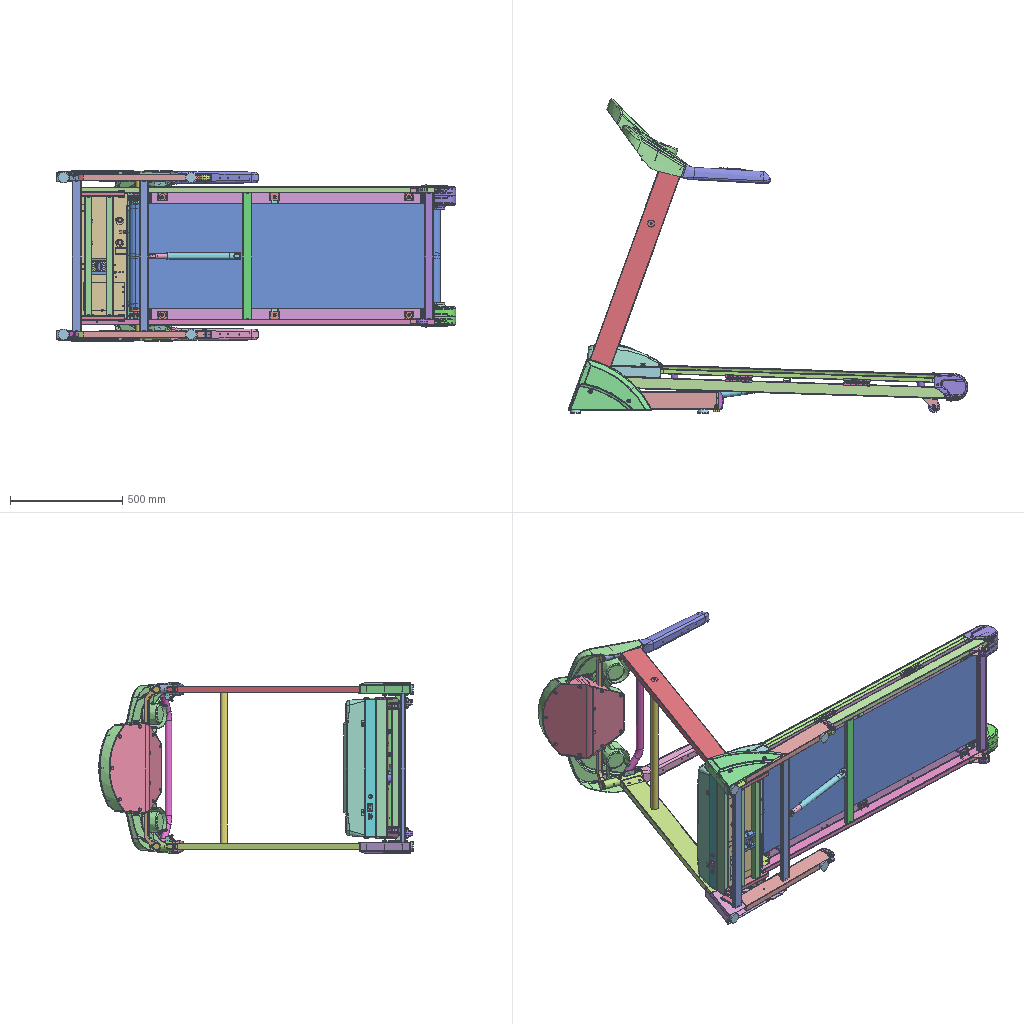Assembly | STEP file | 109 different items | 222 placed | box 1782 x 1401 x 762 mm
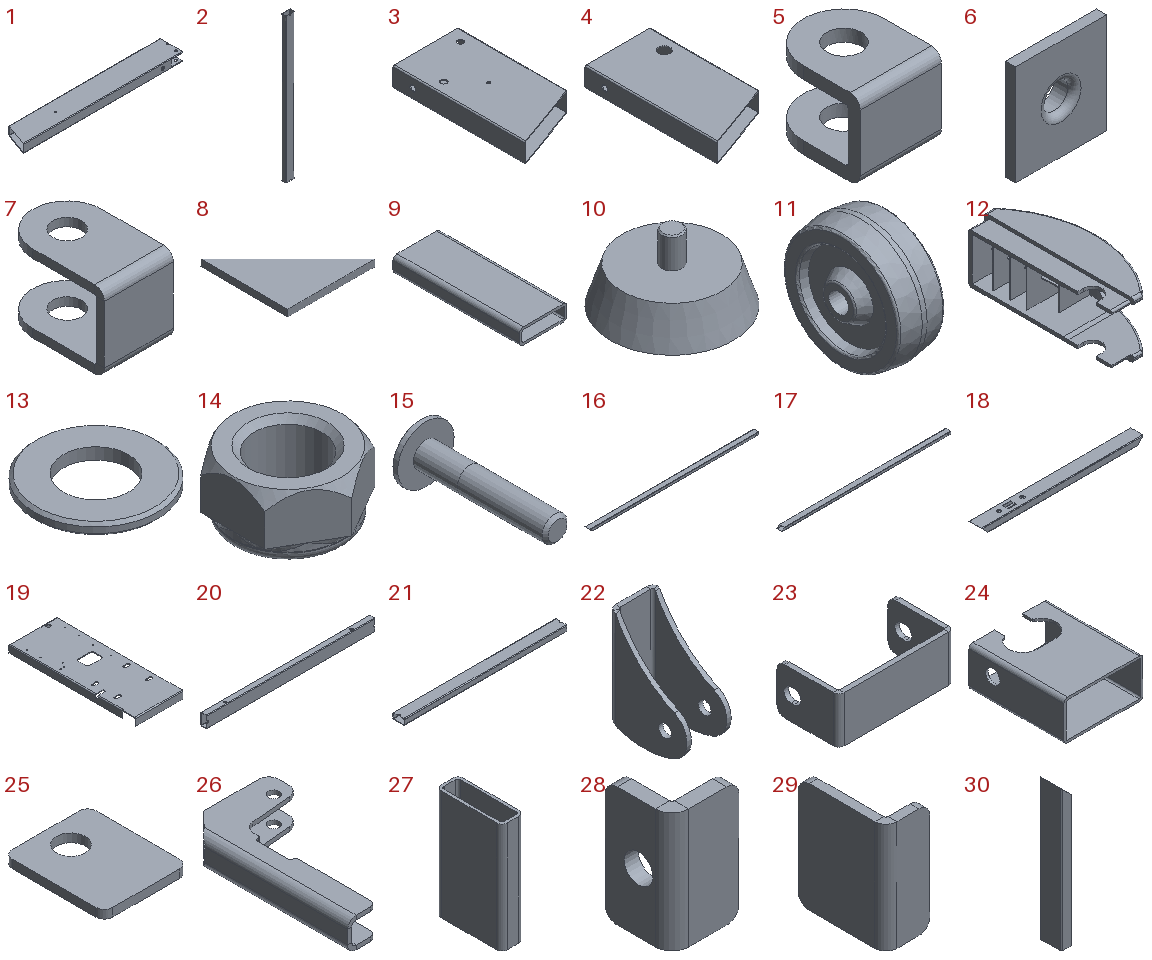Parts list (item | name | quantity | parent item | size | volume):
1 | 7100101 | x2 | in 7100100 | 550 x 80 x 30 mm | 167922 mm3
2 | 7100102 | x2 | in 7100100 | 40 x 20 x 670 mm | 111433 mm3
3 | PN_0021 | x1 | in 7100100 | 100 x 200 x 30 mm | 68376 mm3
4 | PN_0060 | x1 | in 7100100 | 100 x 200 x 30 mm | 68036 mm3
5 | PN_0076_default | x1 | in 7100100 | 20 x 24 x 19 mm | 3011 mm3
6 | 7100105 | x2 | in 7100100 | 27 x 6 x 30 mm | 2422 mm3
7 | 7100106 | x4 | in 7100100, 7100500 | 25 x 38.5 x 28 mm | 6374 mm3
8 | 7100107 | x4 | in 7100100 | 40 x 40 x 3 mm | 2400 mm3
9 | 7100109 | x2 | in 7100100 | 30 x 80 x 10 mm | 8519 mm3
10 | 7100103W | x4 | in PN_0072 | 48.954 x 48.954 x 27.5 mm | 24706 mm3
11 | PN_0027 | x1 | in PN_0072 | 22 x 52.843 x 52.843 mm | 34026 mm3
12 | 7100102W | x2 | in PN_0072 | 30 x 80 x 30 mm | 16145 mm3
13 | PN_0069 | x7 | in PN_0072, PN_0095 | 17 x 17 x 1.6 mm | 252.969 mm3
14 | PN_0039 | x4 | in PN_0072, PN_0095 | 13.017 x 15.011 x 7.5 mm | 666.866 mm3
15 | PN_0065 | x4 | in PN_0072, PN_0095 | 18 x 46.451 x 18 mm | 2805 mm3
16 | PN_0068 | x1 | in 7100500 | 1650 x 50 x 25 mm | 346400 mm3
17 | PN_0073 | x1 | in 7100500 | 1650 x 50 x 25 mm | 346388 mm3
18 | 7100502 | x1 | in 7100500 | 613 x 50 x 25 mm | 116984 mm3
19 | PN_0081_default | x1 | in 7100500 | 210 x 564 x 33 mm | 418851 mm3
20 | 7100504 | x1 | in 7100500 | 565 x 20 x 40 mm | 94145 mm3
21 | 7100505 | x1 | in 7100500 | 565 x 40 x 20 mm | 93951 mm3
22 | 7100506 | x2 | in 7100500 | 30 x 53 x 70.522 mm | 17329 mm3
23 | 7100507 | x2 | in 7100500 | 75 x 40 x 30 mm | 12701 mm3
24 | 7100508 | x1 | in 7100500 | 50 x 60 x 25 mm | 11554 mm3
25 | 7100509 | x1 | in 7100500 | 50 x 60 x 5 mm | 13731 mm3
26 | 7100510 | x1 | in 7100500 | 84 x 160 x 29 mm | 53248 mm3
27 | 7100511 | x2 | in 7100500 | 10 x 30 x 50 mm | 4316 mm3
28 | 7100513 | x4 | in 7100500 | 14 x 14 x 25 mm | 1710 mm3
29 | 7100514 | x2 | in 7100500 | 10 x 20 x 25 mm | 1357 mm3
30 | 7100515 | x1 | in 7100500 | 25 x 50 x 325 mm | 66092 mm3
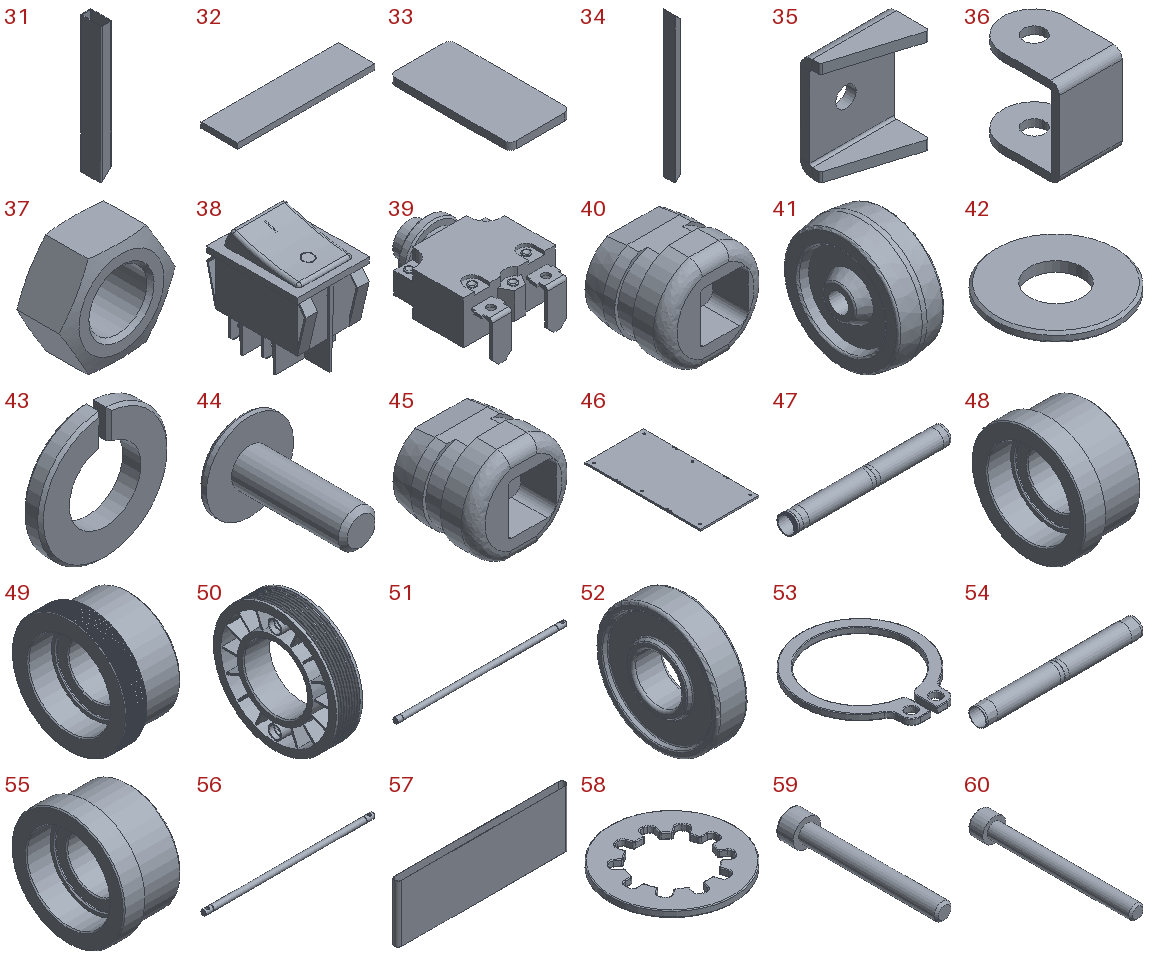31 | 7100516 | x1 | in 7100500 | 25 x 50 x 325 mm | 65710 mm3
32 | 7100517 | x2 | in 7100500 | 75 x 20 x 3 mm | 4500 mm3
33 | 7100518 | x2 | in 7100500 | 25 x 50 x 3 mm | 3734 mm3
34 | 7100519 | x1 | in 7100500 | 25 x 50 x 613 mm | 124358 mm3
35 | 7100520 | x6 | in 7100500 | 35 x 18.649 x 43 mm | 8130 mm3
36 | 7100521 | x1 | in 7100500 | 25 x 35 x 35 mm | 6553 mm3
37 | PN_0091 | x19 | in 7100500, 7101200, PN_0017, PN_0018 | 16 x 7 x 13.856 mm | 779.97 mm3
38 | EP002 | x1 | in PN_0095 | 25 x 34.5 x 34.784 mm | 14567 mm3
39 | EC002 | x1 | in PN_0095 | 29.3 x 39.3 x 19.65 mm | 10331 mm3
40 | PN_0075_default | x1 | in PN_0095 | 17 x 14 x 16 mm | 1519 mm3
41 | PN_0036 | x2 | in PN_0095 | 22 x 52.843 x 52.843 mm | 34026 mm3
42 | PN_0057 | x6 | in PN_0095 | 9.8 x 9.8 x 0.8 mm | 48.045 mm3
43 | PN_0080 | x5 | in PN_0095 | 9.2 x 1.3 x 9.193 mm | 57.255 mm3
44 | PN_0093 | x8 | in PN_0095 | 9.4 x 14.503 x 9.4 mm | 245.335 mm3
45 | PN_0096_default | x1 | in PN_0095 | 17 x 14 x 16 mm | 1519 mm3
46 | DECAK 601 | x1 | in PN_0095 | 605 x 1200 x 18 mm | 13042894 mm3
47 | PN_0083_default | x1 | in PN_0022 | 495 x 56 x 56 mm | 244128 mm3
48 | PN_0001_default | x1 | in PN_0022 | 30 x 55.001 x 55.001 mm | 38129 mm3
49 | PN_0034_default | x1 | in PN_0022 | 30 x 55.999 x 56 mm | 38879 mm3
50 | PN_0025_default | x1 | in PN_0022 | 23 x 108.001 x 108.001 mm | 96628 mm3
51 | 7100702 | x1 | in PN_0038 | 565 x 17 x 17 mm | 128589 mm3
52 | PL6203ZZA_default | x4 | in PN_0038, PN_0026 | 11 x 44 x 44 mm | 11669 mm3
53 | PN_0084 | x4 | in PN_0038, PN_0026 | 19 x 21.5 x 1 mm | 101.865 mm3
54 | PN_0050_default | x1 | in PN_0078 | 485 x 56 x 56 mm | 236794 mm3
55 | PN_0003_default | x2 | in PN_0078 | 30 x 54.43 x 54.43 mm | 37639 mm3
56 | 7100803 | x1 | in PN_0026 | 560 x 17 x 17 mm | 125657 mm3
57 | RUBE 601 | x1 | in PN_0095 | 1389 x 59.2 x 465 mm | 2113671 mm3
58 | PN_0023 | x3 | in PN_0095 | 15 x 15 x 0.8 mm | 82.689 mm3
59 | PN_0020 | x1 | in PN_0095 | 13 x 73 x 13 mm | 4160 mm3
60 | PN_0049 | x2 | in PN_0095 | 13 x 88 x 13 mm | 4914 mm3
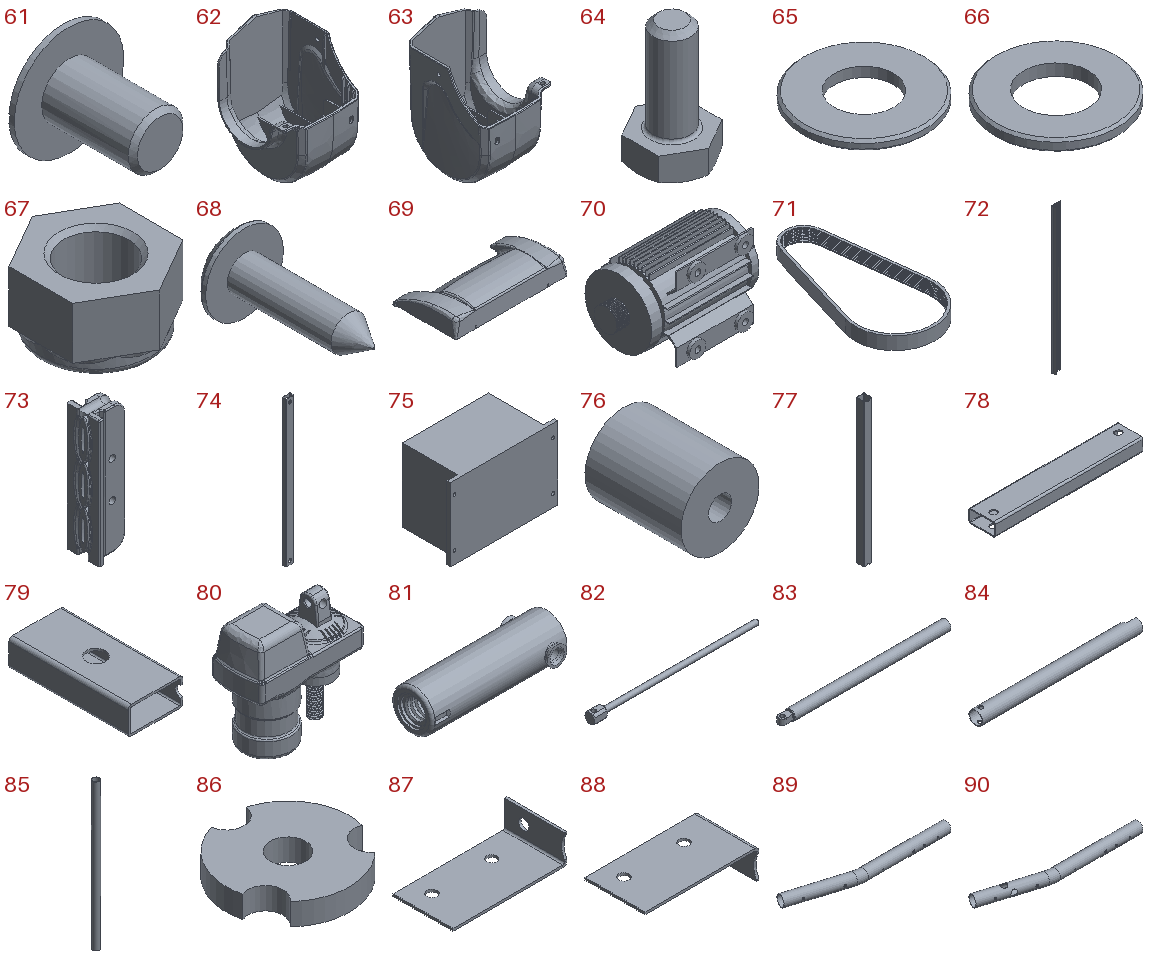61 | PN_0016 | x3 | in PN_0095 | 12 x 12.352 x 12 mm | 428.238 mm3
62 | EDN CAP 601L | x1 | in PN_0095 | - | 183620 mm3
63 | EDN CAP 601R | x1 | in PN_0095 | - | 183322 mm3
64 | PN_0058_M10 | x4 | in PN_0095 | 17 x 19.6 x 32 mm | 3678 mm3
65 | PN_0085 | x4 | in PN_0095 | 25 x 25 x 2 mm | 736.18 mm3
66 | PN_0092 | x4 | in PN_0095 | 21 x 21 x 2 mm | 492.233 mm3
67 | PN_0090 | x4 | in PN_0095 | 17 x 19.63 x 10.5 mm | 1722 mm3
68 | PN_0011 | x2 | in PN_0095 | 9 x 17.646 x 9 mm | 255.973 mm3
69 | 96L | x1 | in PN_0095 | - | -
70 | AC MOTOR 1.5KW | x1 | in PN_0095 | 263.5 x 156.005 x 174 mm | 3095920 mm3
71 | DE200JS8 | x1 | in PN_0095 | 111 x 221.3 x 18 mm | 22925 mm3
72 | SIDE | x2 | in PN_0095 | 76 x 36.5 x 1230 mm | 490001 mm3
73 | jianzhendian | x2 | in PN_0095 | 30 x 30 x 117 mm | 56101 mm3
74 | 7100901 | x1 | in PN_0095 | 30 x 15 x 555 mm | 54621 mm3
75 | Inverter | x1 | in PN_0095 | 185 x 101 x 126 mm | 1922919 mm3
76 | DECH02 | x4 | in PN_0095 | 30 x 37 x 30 mm | 23800 mm3
77 | PN_0043_default | x2 | in 7100400 | 30 x 30 x 532 mm | 88457 mm3
78 | 7100402 | x2 | in 7100400 | 225 x 40 x 20 mm | 36971 mm3
79 | 7100403 | x2 | in 7100400 | 30 x 65 x 15 mm | 6216 mm3
80 | J09 601A_default | x1 | in 710 | 148.1 x 70.5 x 151.812 mm | 777031 mm3
81 | J09 601B | x1 | in 710 | 115 x 41.999 x 35 mm | 49295 mm3
82 | GAS SHOCK 609S | x1 | in 710 | 353.5 x 20 x 20 mm | 34694 mm3
83 | GAS SHOCK 609X | x1 | in 710 | 359 x 22 x 22 mm | 94119 mm3
84 | GAS SHOCK 610W | x1 | in 710 | 330 x 28 x 28 mm | 39789 mm3
85 | 7101301 | x1 | in 7101300 | 31.8 x 31.8 x 725 mm | 103519 mm3
86 | PN_0051_default | x2 | in 7101300 | 28 x 27.429 x 5 mm | 2473 mm3
87 | PN_0007 | x1 | in 7101200 | 95 x 50 x 24.5 mm | 11238 mm3
88 | PN_0031 | x1 | in 7101200 | 95 x 50 x 24.5 mm | 11238 mm3
89 | PN_0002 | x1 | in 7101200 | 530.631 x 103.035 x 38.1 mm | 88866 mm3
90 | PN_0042 | x1 | in 7101200 | 530.631 x 103.035 x 38.1 mm | 88372 mm3
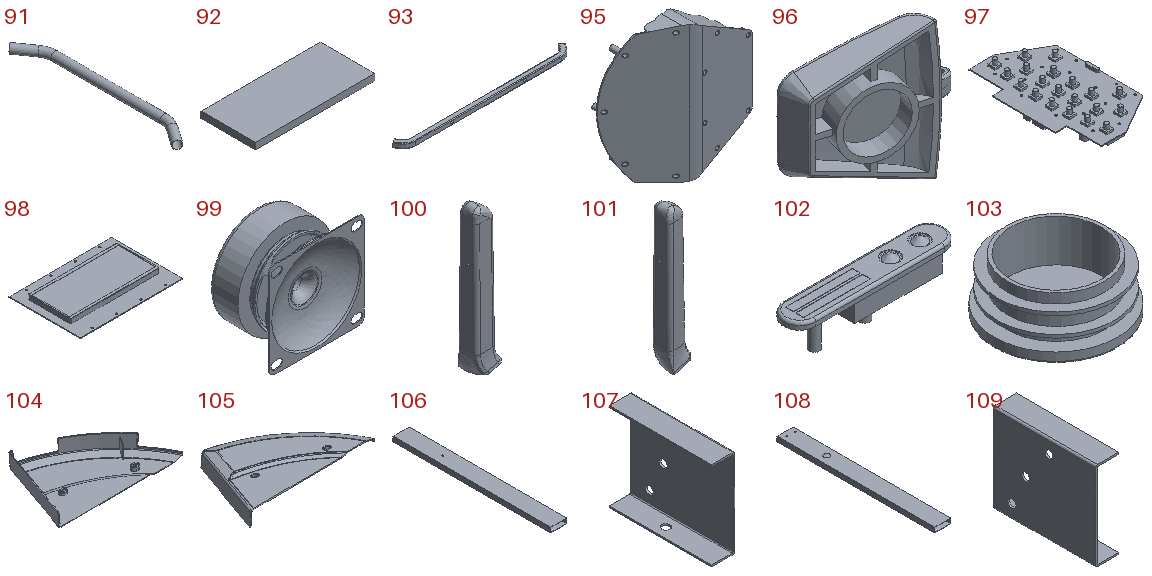91 | 7101203 | x1 | in 7101200 | 89.278 x 660.628 x 31.8 mm | 96707 mm3
92 | 7101204 | x2 | in 7101200 | 55 x 25 x 3 mm | 4125 mm3
93 | 7101205 | x1 | in 7101200 | 697.147 x 49.49 x 20 mm | 75230 mm3
94 | NA609S-A | x1 | in NA609SZ | - | -
95 | NA609S-B | x1 | in NA609SZ | 340.609 x 142.904 x 405.431 mm | 455741 mm3
96 | NA609S-C | x1 | in NA609SZ | 35.148 x 15.37 x 38.312 mm | 3411 mm3
97 | PCB Plate-618 | x1 | in NA609SZ | 132 x 230 x 23.4 mm | 58668 mm3
98 | - | x1 | in NA609SZ | 210 x 145 x 11 mm | 188408 mm3
99 | - | x2 | in NA609SZ | 50 x 31.5 x 50 mm | 33375 mm3
100 | PN_0006 | x1 | in PN_0061 | 71.872 x 63.257 x 397.874 mm | 548309 mm3
101 | PN_0048 | x1 | in PN_0061 | 71.871 x 63.257 x 397.874 mm | 548109 mm3
102 | 7101207W | x2 | in PN_0061 | 119.5 x 24 x 32.509 mm | 28513 mm3
103 | 7101208W | x2 | in PN_0061 | 38 x 38 x 16 mm | 5202 mm3
104 | Right column cover | x1 | in 710 | 372.789 x 229.022 x 48 mm | 179177 mm3
105 | Left column cover | x1 | in 710 | 372.789 x 229.022 x 48 mm | 179176 mm3
106 | PN_0071 | x1 | in PN_0017 | 100 x 950 x 30 mm | 355925 mm3
107 | PN_0066 | x1 | in PN_0017 | 25 x 110 x 95 mm | 29808 mm3
108 | PN_0087 | x1 | in PN_0018 | 100 x 950 x 30 mm | 355925 mm3
109 | PN_0012 | x1 | in PN_0018 | 25 x 110 x 95 mm | 29808 mm3
Placements (level | parent | child | x y z in mm | rotation matrix by rows):
1 | 710 | PN_0072 | 319.734 -99.186 350.0 | 1 0 0 0 1 0 0 0 1
2 | PN_0072 | 7100100 | -0.0 -0.0 -0.0 | 1 0 0 0 1 0 0 0 1
3 | 7100100 | 7100101 | -0.0 -0.0 -0.0 | 1 0 0 0 1 0 0 0 1
3 | 7100100 | 7100101 | -0.0 -0.0 -700.0 | 1 0 0 0 1 0 0 0 1
3 | 7100100 | 7100102 | -280.0 20.0 -350.0 | 1 0 0 0 1 0 0 0 1
3 | 7100100 | 7100102 | -580.0 20.0 -350.0 | 1 0 0 0 1 0 0 0 1
3 | 7100100 | PN_0021 | -609.433 -17.101 -0.0 | 0.9397 0.342 0 -0.342 0.9397 0 0 0 1
3 | 7100100 | PN_0060 | -609.433 -17.101 -700.0 | 0.9397 0.342 0 -0.342 0.9397 0 0 0 1
3 | 7100100 | PN_0076_default | -260.0 30.0 -350.0 | 0 1 0 -1 0 0 0 0 1
3 | 7100100 | 7100105 | -638.73 0.0 0.0 | 0 0 -1 0 1 0 1 0 -0
3 | 7100100 | 7100105 | -638.73 0.0 -700.0 | 0 0 1 0 1 0 -1 0 0
3 | 7100100 | 7100106 | -580.0 40.0 -74.0 | 1 0 0 0 1 0 0 0 1
3 | 7100100 | 7100106 | -580.0 40.0 -626.0 | 1 0 0 0 1 0 0 0 1
3 | 7100100 | 7100107 | -560.0 80.0 -685.0 | 0 0 -1 0 1 0 1 0 0
3 | 7100100 | 7100107 | -563.0 80.0 -15.0 | 0 0 1 0 1 0 -1 0 0
3 | 7100100 | 7100107 | -281.5 80.0 -15.0 | 0 0 1 0 1 0 -1 0 0
3 | 7100100 | 7100107 | -281.5 40.0 -645.0 | 0 0 1 1 0 0 0 1 -0
3 | 7100100 | 7100109 | -599.674 40.0 -672.775 | 1 0 0 0 1 0 0 0 1
3 | 7100100 | 7100109 | -599.674 40.0 -12.775 | 1 0 0 0 1 0 0 0 1
2 | PN_0072 | 7100103W | -638.73 0.0 -0.0 | 0.9991 -0.04147 0 0 0 1 -0.04147 -0.9991 0
2 | PN_0072 | 7100103W | -70.0 -0.0 0.0 | -0.9344 0.3562 0 0 0 1 0.3562 0.9344 0
2 | PN_0072 | PN_0027 | -10.0 15.0 -0.0 | 0 0 1 0 1 0 -1 0 0
2 | PN_0072 | 7100102W | -0.0 40.0 -0.0 | 1 0 0 0 1 0 0 0 1
2 | PN_0072 | PN_0069 | -10.0 15.0 -16.6 | 1 0 0 0 1 0 0 0 1
2 | PN_0072 | PN_0069 | -10.0 15.0 -683.4 | -0.9237 -0.383 0 -0.383 0.9237 0 0 0 -1
2 | PN_0072 | PN_0039 | -10.0 15.0 -22.1 | 1 0 0 0 1 0 0 0 1
2 | PN_0072 | PN_0039 | -10.0 15.0 -677.9 | -0.9237 -0.383 0 -0.383 0.9237 0 0 0 -1
2 | PN_0072 | PN_0065 | -10.0 15.0 15.0 | 1 0 0 0 0 -1 0 1 0
2 | PN_0072 | PN_0065 | -10.0 15.0 -715.0 | 1 0 0 0 0 1 0 -1 0
2 | PN_0072 | 7100103W | -638.73 0.0 -700.0 | 0.9991 -0.04147 0 0 0 1 -0.04147 -0.9991 0
2 | PN_0072 | 7100103W | -70.0 -0.0 -700.0 | -0.9344 0.3562 0 0 0 1 0.3562 0.9344 0
2 | PN_0072 | 7100102W | -0.0 40.0 -700.0 | 1 0 0 0 1 0 0 0 1
1 | 710 | PN_0095 | 446.175 68.129 310.459 | 0.9995 0.03221 0 -0.03221 0.9995 0 0 0 1
2 | PN_0095 | 7100500 | -0.0 -0.0 -0.0 | 1 0 0 0 1 0 0 0 1
3 | 7100500 | PN_0068 | 112.255 -64.436 -15.459 | 1 0 0 0 1 0 0 0 1
3 | 7100500 | PN_0073 | 112.255 -64.436 -605.459 | 1 0 0 0 1 0 0 0 1
3 | 7100500 | 7100502 | -700.245 -14.436 -310.459 | 0 0 -1 0 1 0 1 0 0
3 | 7100500 | PN_0081_default | -687.745 -86.436 -310.459 | -1 0 0 0 0 -1 0 -1 0
3 | 7100500 | 7100504 | 867.255 -79.436 -310.459 | 0 0 1 0 1 0 -1 0 -0
3 | 7100500 | 7100505 | 57.255 -79.436 -310.459 | 0 -1 0 0 0 -1 1 0 0
3 | 7100500 | 7100506 | 825.755 -89.436 -17.959 | 0 0 -1 0 1 0 1 0 0
3 | 7100500 | 7100506 | 825.755 -89.436 -602.959 | 0 0 -1 0 1 0 1 0 0
3 | 7100500 | 7100507 | 899.755 -24.436 -32.959 | 1 0 0 0 0 1 0 -1 0
3 | 7100500 | 7100507 | 899.755 -24.436 -587.959 | 1 0 0 0 0 -1 0 1 -0
3 | 7100500 | 7100508 | -442.745 -39.436 -580.459 | 1 0 0 0 1 0 0 0 1
3 | 7100500 | 7100509 | -442.745 -69.436 -32.959 | 1 0 0 0 1 0 0 0 1
3 | 7100500 | 7100510 | -666.745 73.564 -357.459 | 1 0 0 0 1 0 0 0 1
3 | 7100500 | 7100511 | -505.745 -137.337 -301.977 | 0 0 1 -1 0 0 0 -1 0
3 | 7100500 | 7100511 | -662.745 -25.535 -109.977 | 0 0 -1 1 0 0 0 -1 -0
3 | 7100500 | 7100513 | -465.745 10.564 -614.959 | 0 0 -1 0 1 0 1 0 0
3 | 7100500 | 7100513 | -712.745 10.564 -112.959 | 1 0 0 0 1 0 0 0 1
3 | 7100500 | 7100513 | -465.745 10.564 -5.959 | 0 0 1 0 1 0 -1 0 0
3 | 7100500 | 7100513 | -712.745 10.564 -507.959 | 1 0 0 0 1 0 0 0 1
3 | 7100500 | 7100514 | 849.755 -39.436 -2.959 | 0 0 1 0 1 0 -1 0 -0
3 | 7100500 | 7100514 | 849.755 -39.436 -617.959 | 0 0 -1 0 1 0 1 0 0
3 | 7100500 | 7100515 | -387.745 -14.436 -605.459 | 0 0 -1 0 1 0 1 0 0
3 | 7100500 | 7100516 | -712.745 -14.436 -15.459 | 0 0 1 0 1 0 -1 0 -0
3 | 7100500 | 7100517 | 899.755 -42.436 -37.959 | 1 0 0 0 0 1 0 -1 -0
3 | 7100500 | 7100517 | 899.755 -42.436 -582.959 | 1 0 0 0 0 1 0 -1 0
3 | 7100500 | 7100518 | -384.745 -14.436 -15.459 | 0 0 -1 0 1 0 1 0 0
3 | 7100500 | 7100518 | -387.745 -14.436 -605.459 | 0 0 1 0 1 0 -1 0 -0
3 | 7100500 | 7100519 | -700.245 -64.436 -616.959 | 1 0 0 0 1 0 0 0 1
3 | 7100500 | 7100520 | -322.745 -56.436 -27.959 | 0 0 -1 0 1 0 1 0 0
3 | 7100500 | 7100520 | 777.255 -56.436 -27.959 | 0 0 -1 0 1 0 1 0 0
3 | 7100500 | 7100520 | -322.745 -56.436 -592.959 | 0 0 1 0 1 0 -1 0 -0
3 | 7100500 | 7100520 | 777.255 -56.436 -592.959 | 0 0 1 0 1 0 -1 0 -0
3 | 7100500 | 7100520 | 177.255 -36.436 -592.959 | 0 0 1 0 1 0 -1 0 -0
3 | 7100500 | 7100520 | 177.255 -36.436 -27.959 | 0 0 -1 0 1 0 1 0 -0
3 | 7100500 | 7100521 | 37.255 -81.936 -310.459 | 0 -1 0 1 0 0 0 0 1
3 | 7100500 | 7100106 | -502.745 -89.436 -586.459 | 1 0 0 0 -1 0 0 0 -1
3 | 7100500 | 7100106 | -502.745 -89.436 -34.459 | 1 0 0 0 -1 0 0 0 -1
3 | 7100500 | PN_0091 | -484.245 -80.364 -203.459 | 0 -1 0 0.866 0 -0.5 0.5 0 0.866
3 | 7100500 | PN_0091 | -322.745 -63.936 -47.959 | 0.866 0 -0.5 0 1 0 0.5 0 0.866
3 | 7100500 | PN_0091 | -322.745 -63.936 -572.959 | 0.866 0 -0.5 0 1 0 0.5 0 0.866
3 | 7100500 | PN_0091 | 177.255 -43.936 -47.959 | 0.866 0 -0.5 0 1 0 0.5 0 0.866
3 | 7100500 | PN_0091 | 777.255 -63.936 -47.959 | 0.866 0 -0.5 0 1 0 0.5 0 0.866
3 | 7100500 | PN_0091 | 777.255 -63.936 -572.959 | 0.8429 0 -0.5381 0 1 0 0.5381 0 0.8429
3 | 7100500 | PN_0091 | 177.255 -43.936 -572.959 | 0.866 0 -0.5 0 1 0 0.5 0 0.866
2 | PN_0095 | EP002 | -712.745 -14.186 -485.709 | 0 0 -1 -1 0 0 0 1 0
2 | PN_0095 | EC002 | -655.465 -21.336 -484.294 | 0 -1 0 0 0 -1 1 0 0
2 | PN_0095 | PN_0075_default | -718.245 -14.524 -437.359 | 0 1 0 -1 0 0 0 0 1
2 | PN_0095 | PN_0036 | 837.255 -127.436 -16.959 | 0 0.005777 -1 0 1 0.005777 1 0 0
2 | PN_0095 | PN_0036 | 837.255 -127.436 -601.959 | 0 0.01299 0.9999 0 0.9999 -0.01299 -1 0 0
2 | PN_0095 | PN_0057 | -497.745 -82.636 -532.459 | 1 0 0 0 0 -1 0 1 -0
2 | PN_0095 | PN_0057 | -590.745 -84.436 -552.459 | 1 0 0 0 0 1 0 -1 0
2 | PN_0095 | PN_0057 | -662.745 -86.436 -322.459 | 0.9885 -0.1514 0 0 0 1 -0.1514 -0.9885 0
2 | PN_0095 | PN_0057 | -532.745 -86.436 -382.459 | 1 0 0 0 0 1 0 -1 0
2 | PN_0095 | PN_0057 | -667.745 -84.436 -532.459 | 0.8986 -0.4389 0 0 0 1 -0.4389 -0.8986 0
2 | PN_0095 | PN_0080 | -497.745 -82.636 -532.459 | -0.2314 0 0.9729 0 1 0 -0.9729 0 -0.2314
2 | PN_0095 | PN_0080 | -662.745 -84.336 -322.459 | 0.9816 0 -0.1911 0 -1 0 -0.1911 0 -0.9816
2 | PN_0095 | PN_0080 | -532.745 -84.336 -382.459 | 1 0 0 0 -1 0 0 0 -1
2 | PN_0095 | PN_0080 | -667.745 -82.336 -532.459 | 1 0 0 0 -1 0 0 0 -1
2 | PN_0095 | PN_0093 | -532.745 -84.336 -382.459 | -0.8802 0 -0.4746 0 1 0 0.4746 0 -0.8802
2 | PN_0095 | PN_0093 | -662.745 -84.336 -322.459 | 0.9884 0 0.152 0 1 0 -0.152 0 0.9884
2 | PN_0095 | PN_0093 | -497.745 -81.336 -532.459 | 0.8688 0 -0.4951 0 1 0 0.4951 0 0.8688
2 | PN_0095 | PN_0093 | -532.745 -81.336 -352.459 | -0.4579 0 -0.889 0 1 0 0.889 0 -0.4579
2 | PN_0095 | PN_0057 | -532.745 -83.436 -352.459 | 1 0 0 0 0 1 0 -1 0
2 | PN_0095 | PN_0080 | -532.745 -81.336 -352.459 | 1 0 0 0 -1 0 0 0 -1
2 | PN_0095 | PN_0069 | 837.255 -127.436 -34.559 | 1 0 0 0 1 0 0 0 1
2 | PN_0095 | PN_0069 | 837.255 -127.436 -586.359 | -1 0 0 0 1 0 0 0 -1
2 | PN_0095 | PN_0065 | 837.255 -127.436 -1.959 | 1 0 0 0 0 -1 0 1 -0
2 | PN_0095 | PN_0065 | 837.255 -127.436 -618.959 | 1 0 0 0 0 1 0 -1 -0
2 | PN_0095 | PN_0039 | 837.255 -127.436 -40.059 | 1 0 0 0 1 0 0 0 1
2 | PN_0095 | PN_0039 | 837.255 -127.436 -580.859 | -0.8858 -0.464 0 -0.464 0.8858 0 0 0 -1
2 | PN_0095 | PN_0096_default | -637.579 -94.936 -577.464 | -0.9995 0 -0.03043 0 1 0 0.03043 0 -0.9995
2 | PN_0095 | DECAK 601 | 227.255 -10.436 -310.459 | 0 -1 0 0 0 1 -1 0 0
2 | PN_0095 | PN_0038 | -442.745 -24.436 -299.659 | 0 1 0 0 0 -1 -1 0 -0
3 | PN_0038 | PN_0022 | 0.0 0.0 -0.0 | 1 0 0 0 1 0 0 0 1
4 | PN_0022 | PN_0083_default | -0.0 -0.0 -0.0 | 1 0 0 0 1 0 0 0 1
4 | PN_0022 | PN_0001_default | 257.5 -0.0 0.0 | -1 0 0 0 0.5057 -0.8627 0 -0.8627 -0.5057
4 | PN_0022 | PN_0034_default | -257.5 -0.0 -0.0 | 1 0 0 0 1 0 0 0 1
4 | PN_0022 | PN_0025_default | -257.5 -0.0 -0.0 | 1 0 0 0 1 0 0 0 1
3 | PN_0038 | 7100702 | -1.7 0.0 -0.0 | 1 0 0 0 0 1 0 -1 -0
3 | PN_0038 | PL6203ZZA_default | 246.5 8.5 -0.0 | 1 0 0 0 1 0 0 0 1
3 | PN_0038 | PL6203ZZA_default | -257.5 8.5 -0.0 | 1 0 0 0 1 0 0 0 1
3 | PN_0038 | PN_0084 | 257.6 0.0 -0.0 | 0 0 1 0 1 0 -1 0 -0
3 | PN_0038 | PN_0084 | -258.6 0.0 -0.0 | 0 0 1 0 1 0 -1 0 -0
2 | PN_0095 | PN_0026 | 887.255 -24.436 -309.459 | 0 0 -1 0 1 0 1 0 0
3 | PN_0026 | PN_0078 | 0.0 0.0 0.0 | 1 0 0 0 1 0 0 0 1
4 | PN_0078 | PN_0050_default | -0.0 -0.0 -0.0 | 1 0 0 0 1 0 0 0 1
4 | PN_0078 | PN_0003_default | -252.5 -0.0 0.0 | 1 0 0 0 1 0 0 0 1
4 | PN_0078 | PN_0003_default | 252.5 0.0 0.0 | -1 0 0 0 0.3818 -0.9242 0 -0.9242 -0.3818
3 | PN_0026 | PL6203ZZA_default | -252.5 8.5 -0.0 | 1 0 0 0 1 0 0 0 1
3 | PN_0026 | PL6203ZZA_default | 241.5 8.5 -0.0 | 1 0 0 0 1 0 0 0 1
3 | PN_0026 | PN_0084 | 252.6 0.0 0.0 | 0 0 1 0 1 0 -1 0 0
3 | PN_0026 | PN_0084 | -252.8 -0.0 0.0 | 0 0 -1 0 1 0 1 0 0
3 | PN_0026 | 7100803 | 0.0 0.0 0.0 | 1 0 0 0 1 0 0 0 1
2 | PN_0095 | RUBE 601 | 805.755 -24.436 -310.459 | 1 0 0 0 1 0 0 0 1
2 | PN_0095 | PN_0023 | 938.055 -24.436 -41.959 | 0 0 -1 0 1 0 1 0 -0
2 | PN_0095 | PN_0023 | -468.545 -24.436 -577.959 | 0 0 1 0 1 0 -1 0 0
2 | PN_0095 | PN_0069 | 939.655 -24.436 -41.959 | 0 0 -1 0 1 0 1 0 -0
2 | PN_0095 | PN_0069 | -470.145 -24.436 -577.959 | 0 0 1 0 1 0 -1 0 0
2 | PN_0095 | PN_0020 | -470.145 -24.436 -577.959 | 0 -1 0 1 0 0 0 0 1
2 | PN_0095 | PN_0049 | 939.655 -24.436 -41.959 | 0 1 0 -0.891 0 0.4541 0.4541 0 0.891
2 | PN_0095 | PN_0093 | 890.255 -81.436 -97.959 | 0 1 0 -1 0 0 0 0 1
2 | PN_0095 | PN_0093 | 890.255 -81.436 -522.959 | 0 1 0 -1 0 0 0 0 1
2 | PN_0095 | PN_0016 | -465.745 17.564 -2.079 | 0.9957 0 -0.09225 -0.09225 0 -0.9957 0 1 0
2 | PN_0095 | PN_0016 | -716.625 17.564 -112.959 | 0 -1 0 1 0 0 0 0 1
2 | PN_0095 | PN_0016 | -465.745 17.564 -618.839 | -0.9199 0 0.3922 -0.3922 0 -0.9199 0 -1 -0
2 | PN_0095 | EDN CAP 601L | 824.255 20.504 -42.468 | 0 0 -1 0 1 0 1 0 -0
2 | PN_0095 | EDN CAP 601R | 824.255 20.504 -578.45 | 0 0 -1 0 1 0 1 0 -0
2 | PN_0095 | PN_0023 | 938.055 -24.436 -576.959 | 0 0 -1 0 1 0 1 0 -0
2 | PN_0095 | PN_0069 | 939.655 -24.436 -576.959 | 0 0 -1 0 1 0 1 0 -0
2 | PN_0095 | PN_0049 | 939.655 -24.436 -576.959 | 0 1 0 -0.891 0 0.4541 0.4541 0 0.891
2 | PN_0095 | PN_0058_M10 | -650.245 -96.436 -149.459 | 0.7133 -0.7008 0 0 0 1 -0.7008 -0.7133 -0
2 | PN_0095 | PN_0058_M10 | -650.245 -96.436 -249.459 | -0.1244 0.9922 0 0 0 1 0.9922 0.1244 -0
2 | PN_0095 | PN_0058_M10 | -510.245 -96.436 -149.459 | 0.87 -0.493 0 0 0 1 -0.493 -0.87 -0
2 | PN_0095 | PN_0058_M10 | -510.245 -96.436 -249.459 | 0.4078 -0.9131 0 0 0 1 -0.9131 -0.4078 0
2 | PN_0095 | PN_0085 | -510.245 -84.436 -249.459 | 1 0 0 0 0 -1 0 1 0
2 | PN_0095 | PN_0085 | -510.245 -84.436 -149.459 | 1 0 0 0 0 -1 0 1 0
2 | PN_0095 | PN_0085 | -650.245 -84.436 -249.459 | 1 0 0 0 0 -1 0 1 0
2 | PN_0095 | PN_0085 | -650.245 -84.436 -149.459 | 1 0 0 0 0 -1 0 1 0
2 | PN_0095 | PN_0092 | -650.245 -79.436 -149.459 | 1 0 0 0 0 -1 0 1 0
2 | PN_0095 | PN_0092 | -510.245 -79.436 -249.459 | 1 0 0 0 0 -1 0 1 0
2 | PN_0095 | PN_0092 | -510.245 -79.436 -149.459 | 1 0 0 0 0 -1 0 1 0
2 | PN_0095 | PN_0092 | -650.245 -79.436 -249.459 | 0.697 0.7171 0 0 0 -1 -0.7171 0.697 0
2 | PN_0095 | PN_0090 | -650.245 -71.436 -149.459 | 1 0 0 0 0 -1 0 1 0
2 | PN_0095 | PN_0090 | -650.245 -71.436 -249.459 | 1 0 0 0 0 -1 0 1 0
2 | PN_0095 | PN_0090 | -510.245 -71.436 -149.459 | 1 0 0 0 0 -1 0 1 0
2 | PN_0095 | PN_0090 | -510.245 -71.436 -249.459 | 1 0 0 0 0 -1 0 1 0
2 | PN_0095 | PN_0093 | 912.255 -96.742 -15.459 | 0.3726 0 -0.928 0 -1 0 -0.928 0 -0.3726
2 | PN_0095 | PN_0093 | 912.255 -96.742 -605.459 | -0.0932 0 -0.9956 0 -1 0 -0.9956 0 0.0932
2 | PN_0095 | PN_0011 | 851.255 -29.496 4.041 | 1 0 0 0 0 -1 0 1 -0
2 | PN_0095 | PN_0011 | 851.255 -29.496 -624.959 | 1 0 0 0 0 1 0 -1 -0
2 | PN_0095 | 96L | -545.552 5.354 -310.459 | 0 1 0 0 0 1 1 0 -0
2 | PN_0095 | AC MOTOR 1.5KW | -581.276 -5.436 -40.435 | 0 0 1 0 1 0 -1 0 0
2 | PN_0095 | DE200JS8 | -147.941 454.58 -53.659 | 0.04941 -0.9988 0 0.9988 0.04941 0 0 0 1
2 | PN_0095 | SIDE | 845.255 17.564 0.0413 | 0 0 1 0 1 0 -1 0 0
2 | PN_0095 | SIDE | -384.745 17.564 -620.959 | 0 0 -1 0 1 0 1 0 -0
2 | PN_0095 | jianzhendian | -94.245 -30.366 -13.959 | 0 0 1 0 1 0 -1 0 -0
2 | PN_0095 | jianzhendian | 431.755 -30.366 -13.959 | 0 0 1 0 1 0 -1 0 -0
2 | PN_0095 | 7100901 | 177.255 -26.936 -311.959 | 1 0 0 0 1 0 0 0 1
2 | PN_0095 | Inverter | -564.657 -86.436 -520.108 | 1 0 0 0 1 0 0 0 1
2 | PN_0095 | DECH02 | -322.745 -56.436 -572.959 | 1 0 0 0 1 0 0 0 1
2 | PN_0095 | DECH02 | 777.255 -56.436 -572.959 | 1 0 0 0 1 0 0 0 1
2 | PN_0095 | DECH02 | -322.745 -56.436 -47.959 | 1 0 0 0 1 0 0 0 1
2 | PN_0095 | DECH02 | 777.255 -56.436 -47.959 | 1 0 0 0 1 0 0 0 1
1 | 710 | 7100400 | -112.88 -38.983 -0.0 | 0.9992 0.0393 0 -0.0393 0.9992 0 0 0 1
2 | 7100400 | PN_0043_default | -0.0 -0.0 -0.0 | 1 0 0 0 1 0 0 0 1
2 | 7100400 | PN_0043_default | -95.0 0.0 -0.0 | 1 0 0 0 1 0 0 0 1
2 | 7100400 | 7100402 | -160.0 5.0 276.0 | 1 0 0 0 1 0 0 0 1
2 | 7100400 | 7100402 | -160.0 5.0 -276.0 | 1 0 0 0 1 0 0 0 1
2 | 7100400 | 7100403 | -47.5 0.0 -16.5 | 0 1 0 1 0 0 0 0 -1
2 | 7100400 | 7100403 | -47.5 0.0 -76.5 | 0 -1 0 1 0 0 0 0 1
1 | 710 | J09 601A_default | -167.112 81.691 -46.75 | -0.9984 0 -0.05688 -0.05688 0 0.9984 0 1 -0
1 | 710 | J09 601B | -166.202 65.717 -46.75 | 0.05688 0 -0.9984 -0.9984 0 -0.05688 0 1 0
1 | 710 | GAS SHOCK 609S | 438.484 -17.068 -0.0 | -0.9899 0.1414 0 -0.1414 -0.9899 0 0 0 1
1 | 710 | GAS SHOCK 609X | 267.269 -41.532 0.0 | 0.9899 -0.1414 0 0.1414 0.9899 0 0 0 1
1 | 710 | GAS SHOCK 610W | 468.183 -12.825 -0.0 | -0.9899 -0.1414 0 -0.1414 0.9899 0 0 0 -1
1 | 710 | 7101300 | 19.018 726.679 1.0 | 0.03536 0.9994 0 -0.9994 0.03536 0 0 0 1
2 | 7101300 | 7101301 | -2.788 -0.8012 -0.0 | 1 0 0 0 1 0 0 0 1
2 | 7101300 | PN_0051_default | -2.788 -0.8012 352.5 | -0.8814 -0.4723 0 0.4723 -0.8814 0 0 0 1
2 | 7101300 | PN_0051_default | -2.788 -0.8012 -357.5 | -0.8814 -0.4723 0 0.4723 -0.8814 0 0 0 1
1 | 710 | PN_0061 | 247.775 997.523 -27.882 | 0 -0.02963 0.9996 0 0.9996 0.02963 -1 0 -0
2 | PN_0061 | 7101200 | 304.618 225.035 478.871 | 1 0 0 0 1 0 0 0 1
3 | 7101200 | PN_0007 | -682.5 -278.485 -685.966 | 0 0 -1 0.3697 -0.9291 0 -0.9291 -0.3697 -0
3 | 7101200 | PN_0031 | 17.5 -278.485 -685.966 | 0 0 -1 0.3697 -0.9291 0 -0.9291 -0.3697 -0
3 | 7101200 | PN_0002 | -682.5 -292.615 -224.121 | 0 0 -1 -0.0819 0.9966 0 0.9966 0.0819 -0
3 | 7101200 | PN_0042 | 17.5 -292.615 -224.121 | 0 0 -1 -0.0819 0.9966 0 0.9966 0.0819 -0
3 | 7101200 | 7101203 | -332.5 -243.522 -554.743 | 0 1 0 -0.3697 0 0.9291 0.9291 0 0.3697
3 | 7101200 | 7101204 | 2.216 -250.15 -589.206 | 0 1 0 -0.3697 0 0.9291 0.9291 0 0.3697
3 | 7101200 | 7101204 | -634.874 -250.15 -589.206 | 0 1 0 -0.3697 0 0.9291 0.9291 0 0.3697
3 | 7101200 | 7101205 | -332.5 -142.708 -710.733 | -1 0 0 0 -0.9291 -0.3697 0 -0.3697 0.9291
3 | 7101200 | PN_0091 | 17.0 -265.652 -674.941 | 1 0 0 0 0.3697 0.9291 0 -0.9291 0.3697
3 | 7101200 | PN_0091 | 9.0 -292.64 -607.113 | 0 -1 0 1 0 0 0 0 1
3 | 7101200 | PN_0091 | 9.0 -274.155 -653.57 | 0 -1 0 1 0 0 0 0 1
3 | 7101200 | PN_0091 | -682.0 -265.652 -674.941 | 1 0 0 0 0.3697 0.9291 0 -0.9291 0.3697
3 | 7101200 | PN_0091 | -674.0 -292.64 -607.113 | 0 1 0 -1 0 0 0 0 1
3 | 7101200 | PN_0091 | -674.0 -274.155 -653.57 | 0 1 0 -1 0 0 0 0 1
2 | PN_0061 | NA609SZ | -27.882 -66.903 -94.29 | 0 0 -1 -0.3697 0.9291 0 0.9291 0.3697 -0
3 | NA609SZ | NA609S-A | 0.0 -0.0 -0.0 | 1 0 0 0 1 0 0 0 1
3 | NA609SZ | NA609S-B | 0.0 -0.0 -0.0 | 1 0 0 0 1 0 0 0 1
3 | NA609SZ | NA609S-C | -270.578 24.903 0.0 | 0.9867 -0.1628 0 0.1628 0.9867 0 0 0 1
3 | NA609SZ | PCB Plate-618 | -2.556 71.901 -0.0 | 0.9801 0 0.1984 -0.1984 0 0.9801 0 -1 0
3 | NA609SZ | subassembly 2 | -313.009 166.698 0.0 | 0 -0.9036 0.4284 0 0.4284 0.9036 -1 0 -0
3 | NA609SZ | subassembly 3 | -248.943 137.978 154.433 | -0.8871 -0.4281 -0.1727 0.4202 -0.9037 0.08179 -0.1911 0 0.9816
3 | NA609SZ | subassembly 3 | -248.943 137.978 -154.433 | -0.8871 -0.4281 0.1727 0.4202 -0.9037 -0.08179 0.1911 0 0.9816
2 | PN_0061 | PN_0006 | -377.882 -43.42 -39.258 | 0 -1 0 0.9966 0 -0.0819 0.0819 0 0.9966
2 | PN_0061 | PN_0048 | 322.118 -43.42 -39.258 | 0 -1 0 0.9966 0 -0.0819 0.0819 0 0.9966
2 | PN_0061 | 7101207W | -373.882 -31.842 132.266 | 0 -1 0 0.0819 0 0.9966 -0.9966 0 0.0819
2 | PN_0061 | 7101207W | 316.118 -31.842 132.266 | 0 -1 0 0.0819 0 0.9966 -0.9966 0 0.0819
2 | PN_0061 | 7101208W | 322.118 42.078 -265.948 | 1 0 0 0 0.9291 -0.3697 0 0.3697 0.9291
2 | PN_0061 | 7101208W | -377.882 42.078 -265.948 | 1 0 0 0 0.9291 -0.3697 0 0.3697 0.9291
1 | 710 | Right column cover | -312.982 -92.7 -19.5 | 1 0.008727 0 -0.008727 1 0 0 0 1
1 | 710 | Left column cover | -312.314 -92.7 19.5 | 1 0.008727 0 -0.008727 1 0 0 0 1
1 | 710 | PN_0017 | -221.124 72.122 350.0 | 0.9397 0.342 0 -0.342 0.9397 0 0 0 1
2 | PN_0017 | PN_0071 | -0.0 -0.0 -0.0 | 1 0 0 0 1 0 0 0 1
2 | PN_0017 | PN_0066 | 2.331 30.0 29.783 | 0 0 1 0 -1 0 1 0 0
2 | PN_0017 | PN_0091 | 42.0 -30.0 -0.5 | 0 1 0 -1 0 0 0 0 1
2 | PN_0017 | PN_0091 | 32.5 -20.0 8.0 | 0.383 0 0.9237 -0.9237 0 0.383 0 -1 -0
2 | PN_0017 | PN_0091 | -32.5 -60.0 8.0 | 0 0 1 -1 0 0 0 -1 -0
1 | 710 | PN_0018 | -221.124 72.122 -350.0 | 0.9397 0.342 0 -0.342 0.9397 0 0 0 1
2 | PN_0018 | PN_0087 | -0.0 -0.0 -0.0 | 1 0 0 0 1 0 0 0 1
2 | PN_0018 | PN_0012 | 2.331 30.0 6.783 | 0 0 1 0 -1 0 1 0 -0
2 | PN_0018 | PN_0091 | -42.249 -30.0 0.5 | 0 1 0 -1 0 0 0 0 1
2 | PN_0018 | PN_0091 | 32.5 -20.0 -8.0 | 0.383 0 -0.9237 -0.9237 0 -0.383 0 1 0
2 | PN_0018 | PN_0091 | -32.5 -60.0 -8.0 | 0 0 -1 -1 0 0 0 1 0